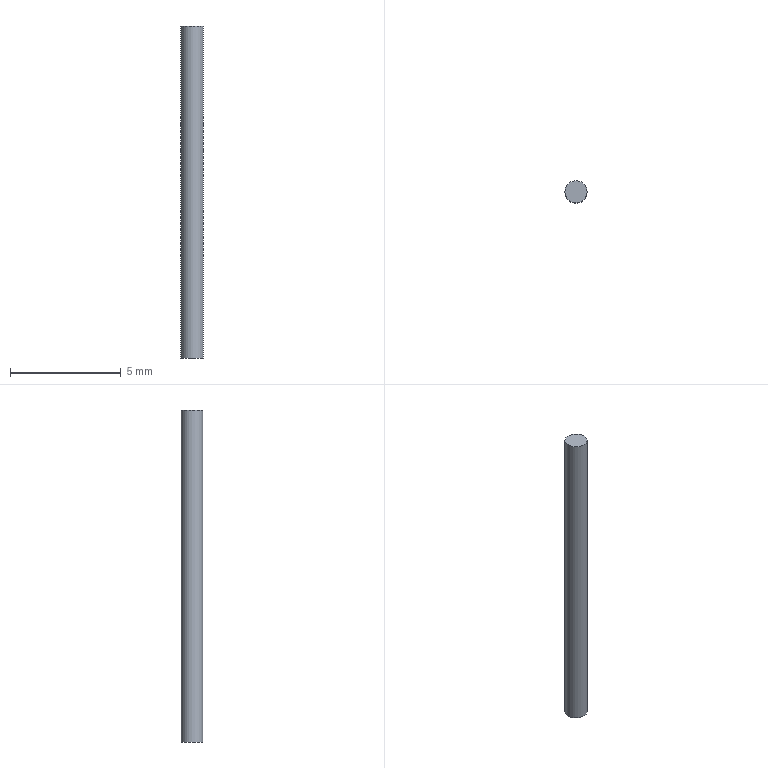Part | NX | 1 solid | 3 faces | box 1 x 1 x 15 mm | volume 11.781 mm3 | plane 2 | cylinder 1 | commonest cylinder face diameters 1 x1
STEP:
#1=CARTESIAN_POINT('',(0.,0.,15.));
#2=VERTEX_POINT('',#1);
#3=CARTESIAN_POINT('',(-0.5,0.,15.));
#4=DIRECTION('',(0.,0.,1.));
#5=DIRECTION('',(1.,0.,0.));
#6=AXIS2_PLACEMENT_3D('',#3,#4,#5);
#7=CIRCLE('',#6,0.5);
#8=EDGE_CURVE('',#2,#2,#7,.F.);
#9=ORIENTED_EDGE('',*,*,#8,.T.);
#10=EDGE_LOOP('',(#9));
#11=FACE_BOUND('',#10,.T.);
#12=CARTESIAN_POINT('',(0.,0.,0.));
#13=VERTEX_POINT('',#12);
#14=CARTESIAN_POINT('',(-0.5,0.,0.));
#15=DIRECTION('',(0.,0.,1.));
#16=DIRECTION('',(1.,0.,0.));
#17=AXIS2_PLACEMENT_3D('',#14,#15,#16);
#18=CIRCLE('',#17,0.5);
#19=EDGE_CURVE('',#13,#13,#18,.T.);
#20=ORIENTED_EDGE('',*,*,#19,.T.);
#21=EDGE_LOOP('',(#20));
#22=FACE_BOUND('',#21,.T.);
#23=CARTESIAN_POINT('',(-0.5,0.,0.));
#24=DIRECTION('',(0.,0.,1.));
#25=DIRECTION('',(1.,0.,0.));
#26=AXIS2_PLACEMENT_3D('',#23,#24,#25);
#27=CYLINDRICAL_SURFACE('',#26,0.5);
#28=ADVANCED_FACE('',(#11,#22),#27,.T.);
#29=ORIENTED_EDGE('',*,*,#19,.F.);
#30=EDGE_LOOP('',(#29));
#31=FACE_BOUND('',#30,.T.);
#32=CARTESIAN_POINT('',(-0.5,0.,0.));
#33=DIRECTION('',(0.,0.,-1.));
#34=DIRECTION('',(-1.,0.,0.));
#35=AXIS2_PLACEMENT_3D('',#32,#33,#34);
#36=PLANE('',#35);
#37=ADVANCED_FACE('',(#31),#36,.T.);
#38=ORIENTED_EDGE('',*,*,#8,.F.);
#39=EDGE_LOOP('',(#38));
#40=FACE_BOUND('',#39,.T.);
#41=CARTESIAN_POINT('',(-0.5,0.,15.));
#42=DIRECTION('',(0.,0.,-1.));
#43=DIRECTION('',(-1.,0.,0.));
#44=AXIS2_PLACEMENT_3D('',#41,#42,#43);
#45=PLANE('',#44);
#46=ADVANCED_FACE('',(#40),#45,.F.);
#47=CLOSED_SHELL('',(#28,#37,#46));
#48=MANIFOLD_SOLID_BREP('',#47);
#49=(LENGTH_UNIT()NAMED_UNIT(*)SI_UNIT(.MILLI.,.METRE.));
#50=UNCERTAINTY_MEASURE_WITH_UNIT(LENGTH_MEASURE(0.00001),#49,'','');
#51=(NAMED_UNIT(*)PLANE_ANGLE_UNIT()SI_UNIT($,.RADIAN.));
#52=(NAMED_UNIT(*)SI_UNIT($,.STERADIAN.)SOLID_ANGLE_UNIT());
#53=(GEOMETRIC_REPRESENTATION_CONTEXT(3)GLOBAL_UNCERTAINTY_ASSIGNED_CONTEXT((#50))GLOBAL_UNIT_ASSIGNED_CONTEXT((#49,#51,#52))REPRESENTATION_CONTEXT('',''));
#54=ADVANCED_BREP_SHAPE_REPRESENTATION('',(#48),#53);